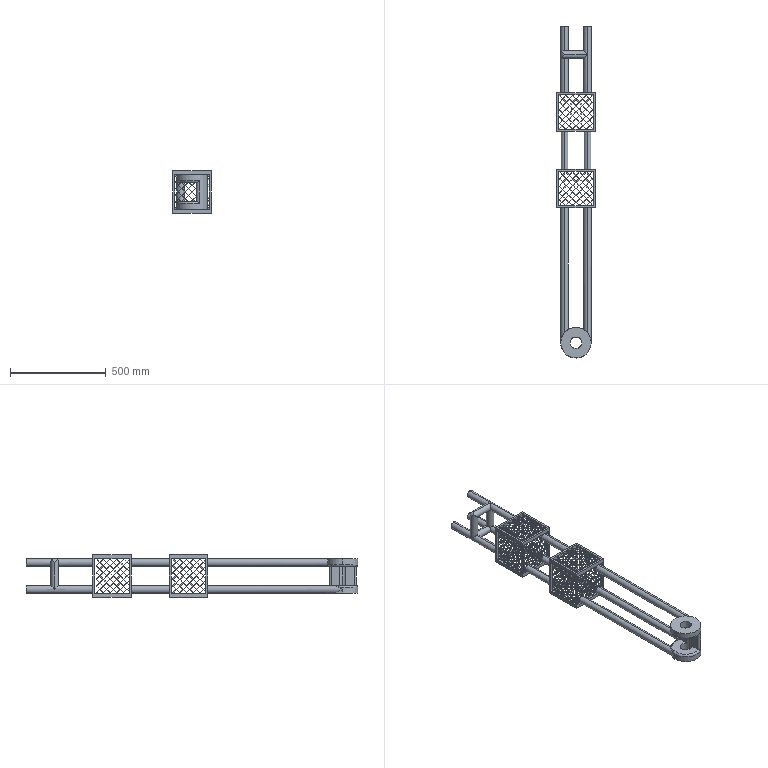Part | SolidWorks | features ICE 8, Cut 6, BossThin 3, MirrorPattern 3, Extrusion 1, Fillet 1, LPattern 1, Sweep 1 | 13 solids | 3254 faces | volume 7988146 mm3 | plane 3197 | cylinder 52 | torus 3 | spline 2 | commonest cylinder face diameters 40 x42 160 x6 20 x2 60 x2